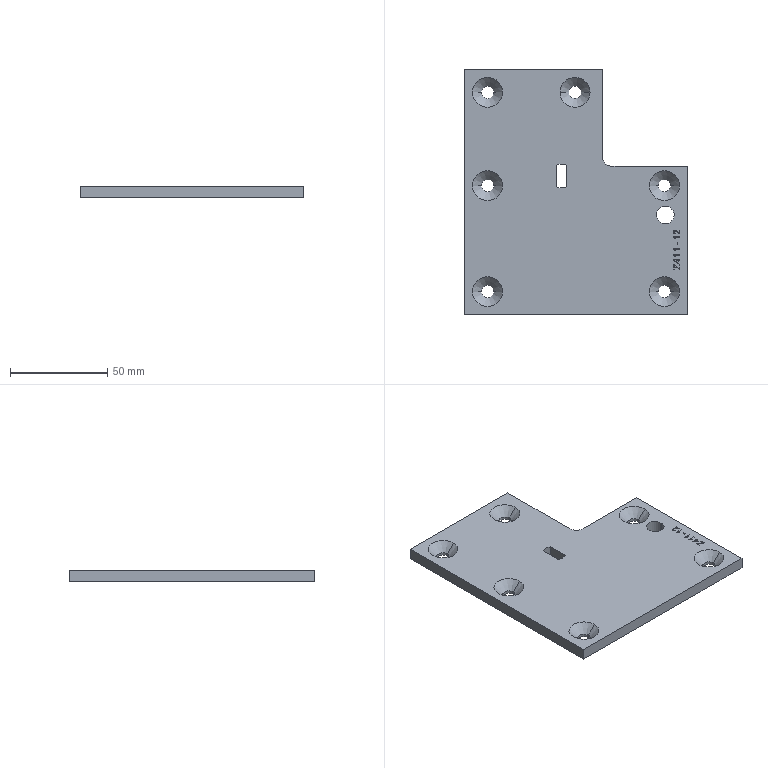Part | Creo | 1 solid | 128 faces | box 115 x 126.5 x 6 mm | volume 70383 mm3 | plane 62 | other 35 | cylinder 19 | cone 12 | commonest cylinder face diameters 6.4 x12 9 x2 12.2 x2 2.89 x1 10 x1 45.582 x1